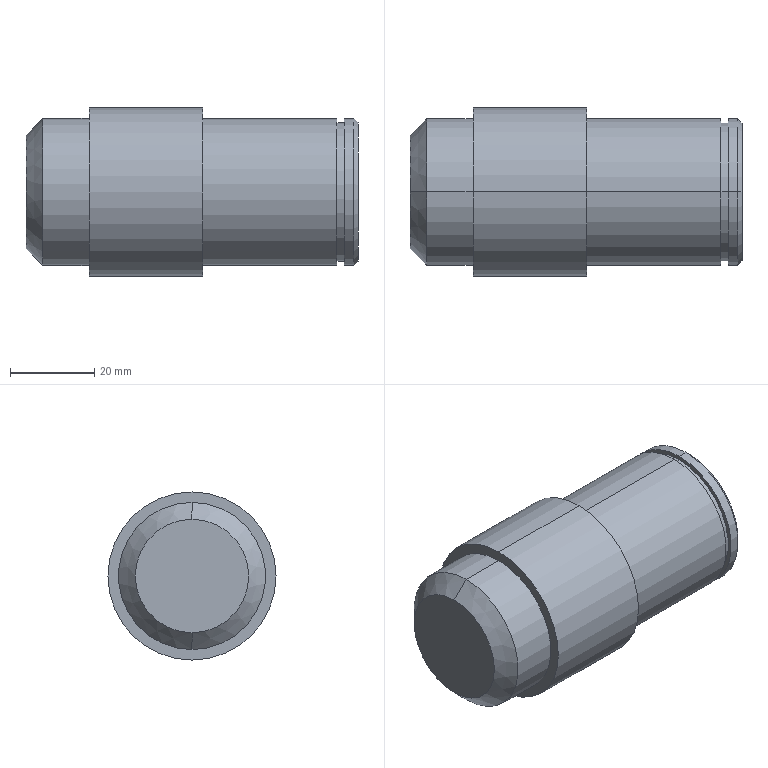Part | STEP file | Driven sprocket shaft | 1 solid | 20 faces | box 79 x 40 x 40 mm | volume 82911 mm3 | cylinder 10 | plane 6 | cone 4 | commonest cylinder face diameters 35 x6 33 x2 40 x2
STEP:
#1=CARTESIAN_POINT('',(0.,0.,0.));
#2=DIRECTION('',(0.,0.,1.));
#3=DIRECTION('',(1.,0.,0.));
#4=AXIS2_PLACEMENT_3D('',#1,#2,#3);
#5=CARTESIAN_POINT('',(0.,0.,13.5));
#6=VERTEX_POINT('',#5);
#7=CARTESIAN_POINT('',(0.,0.,-13.5));
#8=VERTEX_POINT('',#7);
#9=CARTESIAN_POINT('',(0.,0.,0.));
#10=DIRECTION('',(-1.,0.,0.));
#11=DIRECTION('',(0.,0.,-1.));
#12=AXIS2_PLACEMENT_3D('',#9,#10,#11);
#13=CIRCLE('',#12,13.5);
#14=CARTESIAN_POINT('',(0.,0.,0.));
#15=DIRECTION('',(1.,0.,0.));
#16=DIRECTION('',(0.,0.,-1.));
#17=AXIS2_PLACEMENT_3D('',#14,#15,#16);
#18=CONICAL_SURFACE('',#17,13.5,0.7854);
#19=CARTESIAN_POINT('',(6.283,0.));
#20=DIRECTION('',(-1.,0.));
#21=VECTOR('',#20,1.);
#22=LINE('',#19,#21);
#23=(GEOMETRIC_REPRESENTATION_CONTEXT(2)PARAMETRIC_REPRESENTATION_CONTEXT()REPRESENTATION_CONTEXT('',''));
#24=DEFINITIONAL_REPRESENTATION('',(#22),#23);
#25=PCURVE('',#18,#24);
#26=CARTESIAN_POINT('',(0.,0.,0.));
#27=DIRECTION('',(1.,0.,0.));
#28=DIRECTION('',(0.,0.,-1.));
#29=AXIS2_PLACEMENT_3D('',#26,#27,#28);
#30=PLANE('',#29);
#31=CARTESIAN_POINT('',(13.5,0.));
#32=CARTESIAN_POINT('',(13.5,-23.383));
#33=CARTESIAN_POINT('',(-6.75,-11.691));
#34=CARTESIAN_POINT('',(-27.,0.));
#35=CARTESIAN_POINT('',(-6.75,11.691));
#36=CARTESIAN_POINT('',(13.5,23.383));
#37=CARTESIAN_POINT('',(13.5,0.));
#38=(BOUNDED_CURVE()B_SPLINE_CURVE(2,(#31,#32,#33,#34,#35,#36,#37),.UNSPECIFIED.,.T.,.F.)B_SPLINE_CURVE_WITH_KNOTS((1,2,2,2,2,1),(-2.094,0.,2.094,4.189,6.283,8.378),.UNSPECIFIED.)CURVE()GEOMETRIC_REPRESENTATION_ITEM()RATIONAL_B_SPLINE_CURVE((1.,0.5,1.,0.5,1.,0.5,1.))REPRESENTATION_ITEM(''));
#39=(GEOMETRIC_REPRESENTATION_CONTEXT(2)PARAMETRIC_REPRESENTATION_CONTEXT()REPRESENTATION_CONTEXT('',''));
#40=DEFINITIONAL_REPRESENTATION('',(#38),#39);
#41=PCURVE('',#30,#40);
#42=SURFACE_CURVE('',#13,(#25,#41),.PCURVE_S1.);
#43=EDGE_CURVE('',#6,#8,#42,.T.);
#44=ORIENTED_EDGE('',*,*,#43,.F.);
#45=CARTESIAN_POINT('',(4.,0.,17.5));
#46=VERTEX_POINT('',#45);
#47=CARTESIAN_POINT('',(0.,0.,13.5));
#48=DIRECTION('',(0.7071,0.,0.7071));
#49=VECTOR('',#48,1.);
#50=LINE('',#47,#49);
#51=CARTESIAN_POINT('',(3.142,0.));
#52=DIRECTION('',(0.,1.));
#53=VECTOR('',#52,1.);
#54=LINE('',#51,#53);
#55=(GEOMETRIC_REPRESENTATION_CONTEXT(2)PARAMETRIC_REPRESENTATION_CONTEXT()REPRESENTATION_CONTEXT('',''));
#56=DEFINITIONAL_REPRESENTATION('',(#54),#55);
#57=PCURVE('',#18,#56);
#58=CARTESIAN_POINT('',(0.,0.,0.));
#59=DIRECTION('',(1.,0.,0.));
#60=DIRECTION('',(0.,0.,-1.));
#61=AXIS2_PLACEMENT_3D('',#58,#59,#60);
#62=CONICAL_SURFACE('',#61,13.5,0.7854);
#63=CARTESIAN_POINT('',(3.142,0.));
#64=DIRECTION('',(0.,1.));
#65=VECTOR('',#64,1.);
#66=LINE('',#63,#65);
#67=(GEOMETRIC_REPRESENTATION_CONTEXT(2)PARAMETRIC_REPRESENTATION_CONTEXT()REPRESENTATION_CONTEXT('',''));
#68=DEFINITIONAL_REPRESENTATION('',(#66),#67);
#69=PCURVE('',#62,#68);
#70=SURFACE_CURVE('',#50,(#57,#69),.PCURVE_S1.);
#71=EDGE_CURVE('',#6,#46,#70,.T.);
#72=ORIENTED_EDGE('',*,*,#71,.T.);
#73=CARTESIAN_POINT('',(4.,0.,-17.5));
#74=VERTEX_POINT('',#73);
#75=CARTESIAN_POINT('',(4.,0.,0.));
#76=DIRECTION('',(1.,0.,0.));
#77=DIRECTION('',(0.,0.,-1.));
#78=AXIS2_PLACEMENT_3D('',#75,#76,#77);
#79=CIRCLE('',#78,17.5);
#80=CARTESIAN_POINT('',(0.,4.));
#81=DIRECTION('',(1.,0.));
#82=VECTOR('',#81,1.);
#83=LINE('',#80,#82);
#84=(GEOMETRIC_REPRESENTATION_CONTEXT(2)PARAMETRIC_REPRESENTATION_CONTEXT()REPRESENTATION_CONTEXT('',''));
#85=DEFINITIONAL_REPRESENTATION('',(#83),#84);
#86=PCURVE('',#18,#85);
#87=CARTESIAN_POINT('',(-1000.,0.,0.));
#88=DIRECTION('',(-1.,0.,0.));
#89=DIRECTION('',(0.,0.,1.));
#90=AXIS2_PLACEMENT_3D('',#87,#88,#89);
#91=CYLINDRICAL_SURFACE('',#90,17.5);
#92=CARTESIAN_POINT('',(3.142,-1004.));
#93=DIRECTION('',(-1.,0.));
#94=VECTOR('',#93,1.);
#95=LINE('',#92,#94);
#96=(GEOMETRIC_REPRESENTATION_CONTEXT(2)PARAMETRIC_REPRESENTATION_CONTEXT()REPRESENTATION_CONTEXT('',''));
#97=DEFINITIONAL_REPRESENTATION('',(#95),#96);
#98=PCURVE('',#91,#97);
#99=SURFACE_CURVE('',#79,(#86,#98),.PCURVE_S1.);
#100=EDGE_CURVE('',#74,#46,#99,.T.);
#101=ORIENTED_EDGE('',*,*,#100,.F.);
#102=CARTESIAN_POINT('',(0.,0.,-13.5));
#103=DIRECTION('',(0.7071,0.,-0.7071));
#104=VECTOR('',#103,1.);
#105=LINE('',#102,#104);
#106=CARTESIAN_POINT('',(0.,0.));
#107=DIRECTION('',(0.,1.));
#108=VECTOR('',#107,1.);
#109=LINE('',#106,#108);
#110=(GEOMETRIC_REPRESENTATION_CONTEXT(2)PARAMETRIC_REPRESENTATION_CONTEXT()REPRESENTATION_CONTEXT('',''));
#111=DEFINITIONAL_REPRESENTATION('',(#109),#110);
#112=PCURVE('',#18,#111);
#113=CARTESIAN_POINT('',(6.283,0.));
#114=DIRECTION('',(0.,1.));
#115=VECTOR('',#114,1.);
#116=LINE('',#113,#115);
#117=(GEOMETRIC_REPRESENTATION_CONTEXT(2)PARAMETRIC_REPRESENTATION_CONTEXT()REPRESENTATION_CONTEXT('',''));
#118=DEFINITIONAL_REPRESENTATION('',(#116),#117);
#119=PCURVE('',#62,#118);
#120=SURFACE_CURVE('',#105,(#112,#119),.PCURVE_S1.);
#121=EDGE_CURVE('',#8,#74,#120,.T.);
#122=ORIENTED_EDGE('',*,*,#121,.F.);
#123=EDGE_LOOP('',(#44,#72,#101,#122));
#124=FACE_BOUND('',#123,.T.);
#125=ADVANCED_FACE('',(#124),#18,.T.);
#126=CARTESIAN_POINT('',(79.,0.,-16.5));
#127=VERTEX_POINT('',#126);
#128=CARTESIAN_POINT('',(79.,0.,16.5));
#129=VERTEX_POINT('',#128);
#130=CARTESIAN_POINT('',(79.,0.,0.));
#131=DIRECTION('',(1.,0.,0.));
#132=DIRECTION('',(0.,0.,1.));
#133=AXIS2_PLACEMENT_3D('',#130,#131,#132);
#134=CIRCLE('',#133,16.5);
#135=CARTESIAN_POINT('',(78.,0.,0.));
#136=DIRECTION('',(-1.,0.,0.));
#137=DIRECTION('',(0.,0.,1.));
#138=AXIS2_PLACEMENT_3D('',#135,#136,#137);
#139=CONICAL_SURFACE('',#138,17.5,0.7854);
#140=CARTESIAN_POINT('',(6.283,-1.));
#141=DIRECTION('',(-1.,0.));
#142=VECTOR('',#141,1.);
#143=LINE('',#140,#142);
#144=(GEOMETRIC_REPRESENTATION_CONTEXT(2)PARAMETRIC_REPRESENTATION_CONTEXT()REPRESENTATION_CONTEXT('',''));
#145=DEFINITIONAL_REPRESENTATION('',(#143),#144);
#146=PCURVE('',#139,#145);
#147=CARTESIAN_POINT('',(79.,17.5,0.));
#148=DIRECTION('',(-1.,0.,0.));
#149=DIRECTION('',(0.,0.,1.));
#150=AXIS2_PLACEMENT_3D('',#147,#148,#149);
#151=PLANE('',#150);
#152=CARTESIAN_POINT('',(16.5,-17.5));
#153=CARTESIAN_POINT('',(16.5,-46.079));
#154=CARTESIAN_POINT('',(-8.25,-31.789));
#155=CARTESIAN_POINT('',(-33.,-17.5));
#156=CARTESIAN_POINT('',(-8.25,-3.211));
#157=CARTESIAN_POINT('',(16.5,11.079));
#158=CARTESIAN_POINT('',(16.5,-17.5));
#159=(BOUNDED_CURVE()B_SPLINE_CURVE(2,(#152,#153,#154,#155,#156,#157,#158),.UNSPECIFIED.,.T.,.F.)B_SPLINE_CURVE_WITH_KNOTS((1,2,2,2,2,1),(-2.094,0.,2.094,4.189,6.283,8.378),.UNSPECIFIED.)CURVE()GEOMETRIC_REPRESENTATION_ITEM()RATIONAL_B_SPLINE_CURVE((1.,0.5,1.,0.5,1.,0.5,1.))REPRESENTATION_ITEM(''));
#160=(GEOMETRIC_REPRESENTATION_CONTEXT(2)PARAMETRIC_REPRESENTATION_CONTEXT()REPRESENTATION_CONTEXT('',''));
#161=DEFINITIONAL_REPRESENTATION('',(#159),#160);
#162=PCURVE('',#151,#161);
#163=SURFACE_CURVE('',#134,(#146,#162),.PCURVE_S1.);
#164=EDGE_CURVE('',#127,#129,#163,.T.);
#165=ORIENTED_EDGE('',*,*,#164,.F.);
#166=CARTESIAN_POINT('',(78.,0.,-17.5));
#167=VERTEX_POINT('',#166);
#168=CARTESIAN_POINT('',(78.,0.,-17.5));
#169=DIRECTION('',(-0.7071,0.,-0.7071));
#170=VECTOR('',#169,1.);
#171=LINE('',#168,#170);
#172=CARTESIAN_POINT('',(3.142,0.));
#173=DIRECTION('',(0.,1.));
#174=VECTOR('',#173,1.);
#175=LINE('',#172,#174);
#176=(GEOMETRIC_REPRESENTATION_CONTEXT(2)PARAMETRIC_REPRESENTATION_CONTEXT()REPRESENTATION_CONTEXT('',''));
#177=DEFINITIONAL_REPRESENTATION('',(#175),#176);
#178=PCURVE('',#139,#177);
#179=CARTESIAN_POINT('',(78.,0.,0.));
#180=DIRECTION('',(-1.,0.,0.));
#181=DIRECTION('',(0.,0.,1.));
#182=AXIS2_PLACEMENT_3D('',#179,#180,#181);
#183=CONICAL_SURFACE('',#182,17.5,0.7854);
#184=CARTESIAN_POINT('',(3.142,0.));
#185=DIRECTION('',(0.,1.));
#186=VECTOR('',#185,1.);
#187=LINE('',#184,#186);
#188=(GEOMETRIC_REPRESENTATION_CONTEXT(2)PARAMETRIC_REPRESENTATION_CONTEXT()REPRESENTATION_CONTEXT('',''));
#189=DEFINITIONAL_REPRESENTATION('',(#187),#188);
#190=PCURVE('',#183,#189);
#191=SURFACE_CURVE('',#171,(#178,#190),.PCURVE_S1.);
#192=EDGE_CURVE('',#127,#167,#191,.T.);
#193=ORIENTED_EDGE('',*,*,#192,.T.);
#194=CARTESIAN_POINT('',(78.,0.,17.5));
#195=VERTEX_POINT('',#194);
#196=CARTESIAN_POINT('',(78.,0.,0.));
#197=DIRECTION('',(-1.,0.,0.));
#198=DIRECTION('',(0.,0.,1.));
#199=AXIS2_PLACEMENT_3D('',#196,#197,#198);
#200=CIRCLE('',#199,17.5);
#201=CARTESIAN_POINT('',(0.,0.));
#202=DIRECTION('',(1.,0.));
#203=VECTOR('',#202,1.);
#204=LINE('',#201,#203);
#205=(GEOMETRIC_REPRESENTATION_CONTEXT(2)PARAMETRIC_REPRESENTATION_CONTEXT()REPRESENTATION_CONTEXT('',''));
#206=DEFINITIONAL_REPRESENTATION('',(#204),#205);
#207=PCURVE('',#139,#206);
#208=CARTESIAN_POINT('',(-1000.,0.,0.));
#209=DIRECTION('',(-1.,0.,0.));
#210=DIRECTION('',(0.,0.,1.));
#211=AXIS2_PLACEMENT_3D('',#208,#209,#210);
#212=CYLINDRICAL_SURFACE('',#211,17.5);
#213=CARTESIAN_POINT('',(0.,-1078.));
#214=DIRECTION('',(1.,0.));
#215=VECTOR('',#214,1.);
#216=LINE('',#213,#215);
#217=(GEOMETRIC_REPRESENTATION_CONTEXT(2)PARAMETRIC_REPRESENTATION_CONTEXT()REPRESENTATION_CONTEXT('',''));
#218=DEFINITIONAL_REPRESENTATION('',(#216),#217);
#219=PCURVE('',#212,#218);
#220=SURFACE_CURVE('',#200,(#207,#219),.PCURVE_S1.);
#221=EDGE_CURVE('',#195,#167,#220,.T.);
#222=ORIENTED_EDGE('',*,*,#221,.F.);
#223=CARTESIAN_POINT('',(78.,0.,17.5));
#224=DIRECTION('',(-0.7071,0.,0.7071));
#225=VECTOR('',#224,1.);
#226=LINE('',#223,#225);
#227=CARTESIAN_POINT('',(0.,0.));
#228=DIRECTION('',(0.,1.));
#229=VECTOR('',#228,1.);
#230=LINE('',#227,#229);
#231=(GEOMETRIC_REPRESENTATION_CONTEXT(2)PARAMETRIC_REPRESENTATION_CONTEXT()REPRESENTATION_CONTEXT('',''));
#232=DEFINITIONAL_REPRESENTATION('',(#230),#231);
#233=PCURVE('',#139,#232);
#234=CARTESIAN_POINT('',(6.283,0.));
#235=DIRECTION('',(0.,1.));
#236=VECTOR('',#235,1.);
#237=LINE('',#234,#236);
#238=(GEOMETRIC_REPRESENTATION_CONTEXT(2)PARAMETRIC_REPRESENTATION_CONTEXT()REPRESENTATION_CONTEXT('',''));
#239=DEFINITIONAL_REPRESENTATION('',(#237),#238);
#240=PCURVE('',#183,#239);
#241=SURFACE_CURVE('',#226,(#233,#240),.PCURVE_S1.);
#242=EDGE_CURVE('',#129,#195,#241,.T.);
#243=ORIENTED_EDGE('',*,*,#242,.F.);
#244=EDGE_LOOP('',(#165,#193,#222,#243));
#245=FACE_BOUND('',#244,.T.);
#246=ADVANCED_FACE('',(#245),#139,.T.);
#247=ORIENTED_EDGE('',*,*,#221,.T.);
#248=CARTESIAN_POINT('',(75.7,0.,-17.5));
#249=VERTEX_POINT('',#248);
#250=CARTESIAN_POINT('',(-1000.,0.,-17.5));
#251=DIRECTION('',(-1.,0.,0.));
#252=VECTOR('',#251,1.);
#253=LINE('',#250,#252);
#254=CARTESIAN_POINT('',(3.142,0.));
#255=DIRECTION('',(0.,1.));
#256=VECTOR('',#255,1.);
#257=LINE('',#254,#256);
#258=(GEOMETRIC_REPRESENTATION_CONTEXT(2)PARAMETRIC_REPRESENTATION_CONTEXT()REPRESENTATION_CONTEXT('',''));
#259=DEFINITIONAL_REPRESENTATION('',(#257),#258);
#260=PCURVE('',#212,#259);
#261=CARTESIAN_POINT('',(-1000.,0.,0.));
#262=DIRECTION('',(-1.,0.,0.));
#263=DIRECTION('',(0.,0.,1.));
#264=AXIS2_PLACEMENT_3D('',#261,#262,#263);
#265=CYLINDRICAL_SURFACE('',#264,17.5);
#266=CARTESIAN_POINT('',(3.142,0.));
#267=DIRECTION('',(0.,1.));
#268=VECTOR('',#267,1.);
#269=LINE('',#266,#268);
#270=(GEOMETRIC_REPRESENTATION_CONTEXT(2)PARAMETRIC_REPRESENTATION_CONTEXT()REPRESENTATION_CONTEXT('',''));
#271=DEFINITIONAL_REPRESENTATION('',(#269),#270);
#272=PCURVE('',#265,#271);
#273=SURFACE_CURVE('',#253,(#260,#272),.PCURVE_S1.);
#274=EDGE_CURVE('',#167,#249,#273,.T.);
#275=ORIENTED_EDGE('',*,*,#274,.T.);
#276=CARTESIAN_POINT('',(75.7,0.,17.5));
#277=VERTEX_POINT('',#276);
#278=CARTESIAN_POINT('',(75.7,0.,0.));
#279=DIRECTION('',(-1.,0.,0.));
#280=DIRECTION('',(0.,0.,1.));
#281=AXIS2_PLACEMENT_3D('',#278,#279,#280);
#282=CIRCLE('',#281,17.5);
#283=CARTESIAN_POINT('',(0.,-1075.7));
#284=DIRECTION('',(1.,0.));
#285=VECTOR('',#284,1.);
#286=LINE('',#283,#285);
#287=(GEOMETRIC_REPRESENTATION_CONTEXT(2)PARAMETRIC_REPRESENTATION_CONTEXT()REPRESENTATION_CONTEXT('',''));
#288=DEFINITIONAL_REPRESENTATION('',(#286),#287);
#289=PCURVE('',#212,#288);
#290=CARTESIAN_POINT('',(75.7,16.5,0.));
#291=DIRECTION('',(1.,0.,0.));
#292=DIRECTION('',(0.,0.,-1.));
#293=AXIS2_PLACEMENT_3D('',#290,#291,#292);
#294=PLANE('',#293);
#295=CARTESIAN_POINT('',(-17.5,-16.5));
#296=CARTESIAN_POINT('',(-17.5,13.811));
#297=CARTESIAN_POINT('',(8.75,-1.345));
#298=CARTESIAN_POINT('',(35.,-16.5));
#299=CARTESIAN_POINT('',(8.75,-31.655));
#300=CARTESIAN_POINT('',(-17.5,-46.811));
#301=CARTESIAN_POINT('',(-17.5,-16.5));
#302=(BOUNDED_CURVE()B_SPLINE_CURVE(2,(#295,#296,#297,#298,#299,#300,#301),.UNSPECIFIED.,.T.,.F.)B_SPLINE_CURVE_WITH_KNOTS((1,2,2,2,2,1),(-2.094,0.,2.094,4.189,6.283,8.378),.UNSPECIFIED.)CURVE()GEOMETRIC_REPRESENTATION_ITEM()RATIONAL_B_SPLINE_CURVE((1.,0.5,1.,0.5,1.,0.5,1.))REPRESENTATION_ITEM(''));
#303=(GEOMETRIC_REPRESENTATION_CONTEXT(2)PARAMETRIC_REPRESENTATION_CONTEXT()REPRESENTATION_CONTEXT('',''));
#304=DEFINITIONAL_REPRESENTATION('',(#302),#303);
#305=PCURVE('',#294,#304);
#306=SURFACE_CURVE('',#282,(#289,#305),.PCURVE_S1.);
#307=EDGE_CURVE('',#277,#249,#306,.T.);
#308=ORIENTED_EDGE('',*,*,#307,.F.);
#309=CARTESIAN_POINT('',(-1000.,0.,17.5));
#310=DIRECTION('',(-1.,0.,0.));
#311=VECTOR('',#310,1.);
#312=LINE('',#309,#311);
#313=CARTESIAN_POINT('',(0.,0.));
#314=DIRECTION('',(0.,1.));
#315=VECTOR('',#314,1.);
#316=LINE('',#313,#315);
#317=(GEOMETRIC_REPRESENTATION_CONTEXT(2)PARAMETRIC_REPRESENTATION_CONTEXT()REPRESENTATION_CONTEXT('',''));
#318=DEFINITIONAL_REPRESENTATION('',(#316),#317);
#319=PCURVE('',#212,#318);
#320=CARTESIAN_POINT('',(6.283,0.));
#321=DIRECTION('',(0.,1.));
#322=VECTOR('',#321,1.);
#323=LINE('',#320,#322);
#324=(GEOMETRIC_REPRESENTATION_CONTEXT(2)PARAMETRIC_REPRESENTATION_CONTEXT()REPRESENTATION_CONTEXT('',''));
#325=DEFINITIONAL_REPRESENTATION('',(#323),#324);
#326=PCURVE('',#265,#325);
#327=SURFACE_CURVE('',#312,(#319,#326),.PCURVE_S1.);
#328=EDGE_CURVE('',#195,#277,#327,.T.);
#329=ORIENTED_EDGE('',*,*,#328,.F.);
#330=EDGE_LOOP('',(#247,#275,#308,#329));
#331=FACE_BOUND('',#330,.T.);
#332=ADVANCED_FACE('',(#331),#212,.T.);
#333=CARTESIAN_POINT('',(75.7,0.,16.5));
#334=VERTEX_POINT('',#333);
#335=CARTESIAN_POINT('',(75.7,0.,-16.5));
#336=VERTEX_POINT('',#335);
#337=CARTESIAN_POINT('',(75.7,0.,0.));
#338=DIRECTION('',(-1.,0.,0.));
#339=DIRECTION('',(0.,0.,1.));
#340=AXIS2_PLACEMENT_3D('',#337,#338,#339);
#341=CIRCLE('',#340,16.5);
#342=CARTESIAN_POINT('',(-1000.,0.,0.));
#343=DIRECTION('',(-1.,0.,0.));
#344=DIRECTION('',(0.,0.,1.));
#345=AXIS2_PLACEMENT_3D('',#342,#343,#344);
#346=CYLINDRICAL_SURFACE('',#345,16.5);
#347=CARTESIAN_POINT('',(0.,-1075.7));
#348=DIRECTION('',(1.,0.));
#349=VECTOR('',#348,1.);
#350=LINE('',#347,#349);
#351=(GEOMETRIC_REPRESENTATION_CONTEXT(2)PARAMETRIC_REPRESENTATION_CONTEXT()REPRESENTATION_CONTEXT('',''));
#352=DEFINITIONAL_REPRESENTATION('',(#350),#351);
#353=PCURVE('',#346,#352);
#354=CARTESIAN_POINT('',(-16.5,-16.5));
#355=CARTESIAN_POINT('',(-16.5,12.079));
#356=CARTESIAN_POINT('',(8.25,-2.211));
#357=CARTESIAN_POINT('',(33.,-16.5));
#358=CARTESIAN_POINT('',(8.25,-30.789));
#359=CARTESIAN_POINT('',(-16.5,-45.079));
#360=CARTESIAN_POINT('',(-16.5,-16.5));
#361=(BOUNDED_CURVE()B_SPLINE_CURVE(2,(#354,#355,#356,#357,#358,#359,#360),.UNSPECIFIED.,.T.,.F.)B_SPLINE_CURVE_WITH_KNOTS((1,2,2,2,2,1),(-2.094,0.,2.094,4.189,6.283,8.378),.UNSPECIFIED.)CURVE()GEOMETRIC_REPRESENTATION_ITEM()RATIONAL_B_SPLINE_CURVE((1.,0.5,1.,0.5,1.,0.5,1.))REPRESENTATION_ITEM(''));
#362=(GEOMETRIC_REPRESENTATION_CONTEXT(2)PARAMETRIC_REPRESENTATION_CONTEXT()REPRESENTATION_CONTEXT('',''));
#363=DEFINITIONAL_REPRESENTATION('',(#361),#362);
#364=PCURVE('',#294,#363);
#365=SURFACE_CURVE('',#341,(#353,#364),.PCURVE_S1.);
#366=EDGE_CURVE('',#334,#336,#365,.T.);
#367=ORIENTED_EDGE('',*,*,#366,.T.);
#368=CARTESIAN_POINT('',(74.,0.,-16.5));
#369=VERTEX_POINT('',#368);
#370=CARTESIAN_POINT('',(-1000.,0.,-16.5));
#371=DIRECTION('',(-1.,0.,0.));
#372=VECTOR('',#371,1.);
#373=LINE('',#370,#372);
#374=CARTESIAN_POINT('',(3.142,0.));
#375=DIRECTION('',(0.,1.));
#376=VECTOR('',#375,1.);
#377=LINE('',#374,#376);
#378=(GEOMETRIC_REPRESENTATION_CONTEXT(2)PARAMETRIC_REPRESENTATION_CONTEXT()REPRESENTATION_CONTEXT('',''));
#379=DEFINITIONAL_REPRESENTATION('',(#377),#378);
#380=PCURVE('',#346,#379);
#381=CARTESIAN_POINT('',(-1000.,0.,0.));
#382=DIRECTION('',(-1.,0.,0.));
#383=DIRECTION('',(0.,0.,1.));
#384=AXIS2_PLACEMENT_3D('',#381,#382,#383);
#385=CYLINDRICAL_SURFACE('',#384,16.5);
#386=CARTESIAN_POINT('',(3.142,0.));
#387=DIRECTION('',(0.,1.));
#388=VECTOR('',#387,1.);
#389=LINE('',#386,#388);
#390=(GEOMETRIC_REPRESENTATION_CONTEXT(2)PARAMETRIC_REPRESENTATION_CONTEXT()REPRESENTATION_CONTEXT('',''));
#391=DEFINITIONAL_REPRESENTATION('',(#389),#390);
#392=PCURVE('',#385,#391);
#393=SURFACE_CURVE('',#373,(#380,#392),.PCURVE_S1.);
#394=EDGE_CURVE('',#336,#369,#393,.T.);
#395=ORIENTED_EDGE('',*,*,#394,.T.);
#396=CARTESIAN_POINT('',(74.,0.,16.5));
#397=VERTEX_POINT('',#396);
#398=CARTESIAN_POINT('',(74.,0.,0.));
#399=DIRECTION('',(-1.,0.,0.));
#400=DIRECTION('',(0.,0.,1.));
#401=AXIS2_PLACEMENT_3D('',#398,#399,#400);
#402=CIRCLE('',#401,16.5);
#403=CARTESIAN_POINT('',(0.,-1074.));
#404=DIRECTION('',(1.,0.));
#405=VECTOR('',#404,1.);
#406=LINE('',#403,#405);
#407=(GEOMETRIC_REPRESENTATION_CONTEXT(2)PARAMETRIC_REPRESENTATION_CONTEXT()REPRESENTATION_CONTEXT('',''));
#408=DEFINITIONAL_REPRESENTATION('',(#406),#407);
#409=PCURVE('',#346,#408);
#410=CARTESIAN_POINT('',(74.,17.5,0.));
#411=DIRECTION('',(-1.,0.,0.));
#412=DIRECTION('',(0.,0.,1.));
#413=AXIS2_PLACEMENT_3D('',#410,#411,#412);
#414=PLANE('',#413);
#415=CARTESIAN_POINT('',(0.,-17.5));
#416=DIRECTION('',(1.,0.));
#417=AXIS2_PLACEMENT_2D('',#415,#416);
#418=CIRCLE('',#417,16.5);
#419=(GEOMETRIC_REPRESENTATION_CONTEXT(2)PARAMETRIC_REPRESENTATION_CONTEXT()REPRESENTATION_CONTEXT('',''));
#420=DEFINITIONAL_REPRESENTATION('',(#418),#419);
#421=PCURVE('',#414,#420);
#422=SURFACE_CURVE('',#402,(#409,#421),.PCURVE_S1.);
#423=EDGE_CURVE('',#397,#369,#422,.T.);
#424=ORIENTED_EDGE('',*,*,#423,.F.);
#425=CARTESIAN_POINT('',(-1000.,0.,16.5));
#426=DIRECTION('',(-1.,0.,0.));
#427=VECTOR('',#426,1.);
#428=LINE('',#425,#427);
#429=CARTESIAN_POINT('',(0.,0.));
#430=DIRECTION('',(0.,1.));
#431=VECTOR('',#430,1.);
#432=LINE('',#429,#431);
#433=(GEOMETRIC_REPRESENTATION_CONTEXT(2)PARAMETRIC_REPRESENTATION_CONTEXT()REPRESENTATION_CONTEXT('',''));
#434=DEFINITIONAL_REPRESENTATION('',(#432),#433);
#435=PCURVE('',#346,#434);
#436=CARTESIAN_POINT('',(6.283,0.));
#437=DIRECTION('',(0.,1.));
#438=VECTOR('',#437,1.);
#439=LINE('',#436,#438);
#440=(GEOMETRIC_REPRESENTATION_CONTEXT(2)PARAMETRIC_REPRESENTATION_CONTEXT()REPRESENTATION_CONTEXT('',''));
#441=DEFINITIONAL_REPRESENTATION('',(#439),#440);
#442=PCURVE('',#385,#441);
#443=SURFACE_CURVE('',#428,(#435,#442),.PCURVE_S1.);
#444=EDGE_CURVE('',#334,#397,#443,.T.);
#445=ORIENTED_EDGE('',*,*,#444,.F.);
#446=EDGE_LOOP('',(#367,#395,#424,#445));
#447=FACE_BOUND('',#446,.T.);
#448=ADVANCED_FACE('',(#447),#346,.T.);
#449=CARTESIAN_POINT('',(74.,0.,17.5));
#450=VERTEX_POINT('',#449);
#451=CARTESIAN_POINT('',(74.,0.,-17.5));
#452=VERTEX_POINT('',#451);
#453=CARTESIAN_POINT('',(74.,0.,0.));
#454=DIRECTION('',(-1.,0.,0.));
#455=DIRECTION('',(0.,0.,1.));
#456=AXIS2_PLACEMENT_3D('',#453,#454,#455);
#457=CIRCLE('',#456,17.5);
#458=CARTESIAN_POINT('',(-1000.,0.,0.));
#459=DIRECTION('',(-1.,0.,0.));
#460=DIRECTION('',(0.,0.,1.));
#461=AXIS2_PLACEMENT_3D('',#458,#459,#460);
#462=CYLINDRICAL_SURFACE('',#461,17.5);
#463=CARTESIAN_POINT('',(0.,-1074.));
#464=DIRECTION('',(1.,0.));
#465=VECTOR('',#464,1.);
#466=LINE('',#463,#465);
#467=(GEOMETRIC_REPRESENTATION_CONTEXT(2)PARAMETRIC_REPRESENTATION_CONTEXT()REPRESENTATION_CONTEXT('',''));
#468=DEFINITIONAL_REPRESENTATION('',(#466),#467);
#469=PCURVE('',#462,#468);
#470=CARTESIAN_POINT('',(0.,-17.5));
#471=DIRECTION('',(1.,0.));
#472=AXIS2_PLACEMENT_2D('',#470,#471);
#473=CIRCLE('',#472,17.5);
#474=(GEOMETRIC_REPRESENTATION_CONTEXT(2)PARAMETRIC_REPRESENTATION_CONTEXT()REPRESENTATION_CONTEXT('',''));
#475=DEFINITIONAL_REPRESENTATION('',(#473),#474);
#476=PCURVE('',#414,#475);
#477=SURFACE_CURVE('',#457,(#469,#476),.PCURVE_S1.);
#478=EDGE_CURVE('',#450,#452,#477,.T.);
#479=ORIENTED_EDGE('',*,*,#478,.T.);
#480=CARTESIAN_POINT('',(42.,0.,-17.5));
#481=VERTEX_POINT('',#480);
#482=CARTESIAN_POINT('',(-1000.,0.,-17.5));
#483=DIRECTION('',(-1.,0.,0.));
#484=VECTOR('',#483,1.);
#485=LINE('',#482,#484);
#486=CARTESIAN_POINT('',(3.142,0.));
#487=DIRECTION('',(0.,1.));
#488=VECTOR('',#487,1.);
#489=LINE('',#486,#488);
#490=(GEOMETRIC_REPRESENTATION_CONTEXT(2)PARAMETRIC_REPRESENTATION_CONTEXT()REPRESENTATION_CONTEXT('',''));
#491=DEFINITIONAL_REPRESENTATION('',(#489),#490);
#492=PCURVE('',#462,#491);
#493=CARTESIAN_POINT('',(-1000.,0.,0.));
#494=DIRECTION('',(-1.,0.,0.));
#495=DIRECTION('',(0.,0.,1.));
#496=AXIS2_PLACEMENT_3D('',#493,#494,#495);
#497=CYLINDRICAL_SURFACE('',#496,17.5);
#498=CARTESIAN_POINT('',(3.142,0.));
#499=DIRECTION('',(0.,1.));
#500=VECTOR('',#499,1.);
#501=LINE('',#498,#500);
#502=(GEOMETRIC_REPRESENTATION_CONTEXT(2)PARAMETRIC_REPRESENTATION_CONTEXT()REPRESENTATION_CONTEXT('',''));
#503=DEFINITIONAL_REPRESENTATION('',(#501),#502);
#504=PCURVE('',#497,#503);
#505=SURFACE_CURVE('',#485,(#492,#504),.PCURVE_S1.);
#506=EDGE_CURVE('',#452,#481,#505,.T.);
#507=ORIENTED_EDGE('',*,*,#506,.T.);
#508=CARTESIAN_POINT('',(42.,0.,17.5));
#509=VERTEX_POINT('',#508);
#510=CARTESIAN_POINT('',(42.,0.,0.));
#511=DIRECTION('',(-1.,0.,0.));
#512=DIRECTION('',(0.,0.,1.));
#513=AXIS2_PLACEMENT_3D('',#510,#511,#512);
#514=CIRCLE('',#513,17.5);
#515=CARTESIAN_POINT('',(0.,-1042.));
#516=DIRECTION('',(1.,0.));
#517=VECTOR('',#516,1.);
#518=LINE('',#515,#517);
#519=(GEOMETRIC_REPRESENTATION_CONTEXT(2)PARAMETRIC_REPRESENTATION_CONTEXT()REPRESENTATION_CONTEXT('',''));
#520=DEFINITIONAL_REPRESENTATION('',(#518),#519);
#521=PCURVE('',#462,#520);
#522=CARTESIAN_POINT('',(42.,20.,0.));
#523=DIRECTION('',(-1.,0.,0.));
#524=DIRECTION('',(0.,0.,1.));
#525=AXIS2_PLACEMENT_3D('',#522,#523,#524);
#526=PLANE('',#525);
#527=CARTESIAN_POINT('',(0.,-20.));
#528=DIRECTION('',(1.,0.));
#529=AXIS2_PLACEMENT_2D('',#527,#528);
#530=CIRCLE('',#529,17.5);
#531=(GEOMETRIC_REPRESENTATION_CONTEXT(2)PARAMETRIC_REPRESENTATION_CONTEXT()REPRESENTATION_CONTEXT('',''));
#532=DEFINITIONAL_REPRESENTATION('',(#530),#531);
#533=PCURVE('',#526,#532);
#534=SURFACE_CURVE('',#514,(#521,#533),.PCURVE_S1.);
#535=EDGE_CURVE('',#509,#481,#534,.T.);
#536=ORIENTED_EDGE('',*,*,#535,.F.);
#537=CARTESIAN_POINT('',(-1000.,0.,17.5));
#538=DIRECTION('',(-1.,0.,0.));
#539=VECTOR('',#538,1.);
#540=LINE('',#537,#539);
#541=CARTESIAN_POINT('',(0.,0.));
#542=DIRECTION('',(0.,1.));
#543=VECTOR('',#542,1.);
#544=LINE('',#541,#543);
#545=(GEOMETRIC_REPRESENTATION_CONTEXT(2)PARAMETRIC_REPRESENTATION_CONTEXT()REPRESENTATION_CONTEXT('',''));
#546=DEFINITIONAL_REPRESENTATION('',(#544),#545);
#547=PCURVE('',#462,#546);
#548=CARTESIAN_POINT('',(6.283,0.));
#549=DIRECTION('',(0.,1.));
#550=VECTOR('',#549,1.);
#551=LINE('',#548,#550);
#552=(GEOMETRIC_REPRESENTATION_CONTEXT(2)PARAMETRIC_REPRESENTATION_CONTEXT()REPRESENTATION_CONTEXT('',''));
#553=DEFINITIONAL_REPRESENTATION('',(#551),#552);
#554=PCURVE('',#497,#553);
#555=SURFACE_CURVE('',#540,(#547,#554),.PCURVE_S1.);
#556=EDGE_CURVE('',#450,#509,#555,.T.);
#557=ORIENTED_EDGE('',*,*,#556,.F.);
#558=EDGE_LOOP('',(#479,#507,#536,#557));
#559=FACE_BOUND('',#558,.T.);
#560=ADVANCED_FACE('',(#559),#462,.T.);
#561=CARTESIAN_POINT('',(42.,0.,20.));
#562=VERTEX_POINT('',#561);
#563=CARTESIAN_POINT('',(42.,0.,-20.));
#564=VERTEX_POINT('',#563);
#565=CARTESIAN_POINT('',(42.,0.,0.));
#566=DIRECTION('',(-1.,0.,0.));
#567=DIRECTION('',(0.,0.,1.));
#568=AXIS2_PLACEMENT_3D('',#565,#566,#567);
#569=CIRCLE('',#568,20.);
#570=CARTESIAN_POINT('',(-1000.,0.,0.));
#571=DIRECTION('',(-1.,0.,0.));
#572=DIRECTION('',(0.,0.,1.));
#573=AXIS2_PLACEMENT_3D('',#570,#571,#572);
#574=CYLINDRICAL_SURFACE('',#573,20.);
#575=CARTESIAN_POINT('',(0.,-1042.));
#576=DIRECTION('',(1.,0.));
#577=VECTOR('',#576,1.);
#578=LINE('',#575,#577);
#579=(GEOMETRIC_REPRESENTATION_CONTEXT(2)PARAMETRIC_REPRESENTATION_CONTEXT()REPRESENTATION_CONTEXT('',''));
#580=DEFINITIONAL_REPRESENTATION('',(#578),#579);
#581=PCURVE('',#574,#580);
#582=CARTESIAN_POINT('',(0.,-20.));
#583=DIRECTION('',(1.,0.));
#584=AXIS2_PLACEMENT_2D('',#582,#583);
#585=CIRCLE('',#584,20.);
#586=(GEOMETRIC_REPRESENTATION_CONTEXT(2)PARAMETRIC_REPRESENTATION_CONTEXT()REPRESENTATION_CONTEXT('',''));
#587=DEFINITIONAL_REPRESENTATION('',(#585),#586);
#588=PCURVE('',#526,#587);
#589=SURFACE_CURVE('',#569,(#581,#588),.PCURVE_S1.);
#590=EDGE_CURVE('',#562,#564,#589,.T.);
#591=ORIENTED_EDGE('',*,*,#590,.T.);
#592=CARTESIAN_POINT('',(15.,0.,-20.));
#593=VERTEX_POINT('',#592);
#594=CARTESIAN_POINT('',(-1000.,0.,-20.));
#595=DIRECTION('',(-1.,0.,0.));
#596=VECTOR('',#595,1.);
#597=LINE('',#594,#596);
#598=CARTESIAN_POINT('',(3.142,0.));
#599=DIRECTION('',(0.,1.));
#600=VECTOR('',#599,1.);
#601=LINE('',#598,#600);
#602=(GEOMETRIC_REPRESENTATION_CONTEXT(2)PARAMETRIC_REPRESENTATION_CONTEXT()REPRESENTATION_CONTEXT('',''));
#603=DEFINITIONAL_REPRESENTATION('',(#601),#602);
#604=PCURVE('',#574,#603);
#605=CARTESIAN_POINT('',(-1000.,0.,0.));
#606=DIRECTION('',(-1.,0.,0.));
#607=DIRECTION('',(0.,0.,1.));
#608=AXIS2_PLACEMENT_3D('',#605,#606,#607);
#609=CYLINDRICAL_SURFACE('',#608,20.);
#610=CARTESIAN_POINT('',(3.142,0.));
#611=DIRECTION('',(0.,1.));
#612=VECTOR('',#611,1.);
#613=LINE('',#610,#612);
#614=(GEOMETRIC_REPRESENTATION_CONTEXT(2)PARAMETRIC_REPRESENTATION_CONTEXT()REPRESENTATION_CONTEXT('',''));
#615=DEFINITIONAL_REPRESENTATION('',(#613),#614);
#616=PCURVE('',#609,#615);
#617=SURFACE_CURVE('',#597,(#604,#616),.PCURVE_S1.);
#618=EDGE_CURVE('',#564,#593,#617,.T.);
#619=ORIENTED_EDGE('',*,*,#618,.T.);
#620=CARTESIAN_POINT('',(15.,0.,20.));
#621=VERTEX_POINT('',#620);
#622=CARTESIAN_POINT('',(15.,0.,0.));
#623=DIRECTION('',(-1.,0.,0.));
#624=DIRECTION('',(0.,0.,1.));
#625=AXIS2_PLACEMENT_3D('',#622,#623,#624);
#626=CIRCLE('',#625,20.);
#627=CARTESIAN_POINT('',(0.,-1015.));
#628=DIRECTION('',(1.,0.));
#629=VECTOR('',#628,1.);
#630=LINE('',#627,#629);
#631=(GEOMETRIC_REPRESENTATION_CONTEXT(2)PARAMETRIC_REPRESENTATION_CONTEXT()REPRESENTATION_CONTEXT('',''));
#632=DEFINITIONAL_REPRESENTATION('',(#630),#631);
#633=PCURVE('',#574,#632);
#634=CARTESIAN_POINT('',(15.,17.5,0.));
#635=DIRECTION('',(1.,0.,0.));
#636=DIRECTION('',(0.,0.,-1.));
#637=AXIS2_PLACEMENT_3D('',#634,#635,#636);
#638=PLANE('',#637);
#639=CARTESIAN_POINT('',(-20.,-17.5));
#640=CARTESIAN_POINT('',(-20.,17.141));
#641=CARTESIAN_POINT('',(10.,-0.1795));
#642=CARTESIAN_POINT('',(40.,-17.5));
#643=CARTESIAN_POINT('',(10.,-34.821));
#644=CARTESIAN_POINT('',(-20.,-52.141));
#645=CARTESIAN_POINT('',(-20.,-17.5));
#646=(BOUNDED_CURVE()B_SPLINE_CURVE(2,(#639,#640,#641,#642,#643,#644,#645),.UNSPECIFIED.,.T.,.F.)B_SPLINE_CURVE_WITH_KNOTS((1,2,2,2,2,1),(-2.094,0.,2.094,4.189,6.283,8.378),.UNSPECIFIED.)CURVE()GEOMETRIC_REPRESENTATION_ITEM()RATIONAL_B_SPLINE_CURVE((1.,0.5,1.,0.5,1.,0.5,1.))REPRESENTATION_ITEM(''));
#647=(GEOMETRIC_REPRESENTATION_CONTEXT(2)PARAMETRIC_REPRESENTATION_CONTEXT()REPRESENTATION_CONTEXT('',''));
#648=DEFINITIONAL_REPRESENTATION('',(#646),#647);
#649=PCURVE('',#638,#648);
#650=SURFACE_CURVE('',#626,(#633,#649),.PCURVE_S1.);
#651=EDGE_CURVE('',#621,#593,#650,.T.);
#652=ORIENTED_EDGE('',*,*,#651,.F.);
#653=CARTESIAN_POINT('',(-1000.,0.,20.));
#654=DIRECTION('',(-1.,0.,0.));
#655=VECTOR('',#654,1.);
#656=LINE('',#653,#655);
#657=CARTESIAN_POINT('',(0.,0.));
#658=DIRECTION('',(0.,1.));
#659=VECTOR('',#658,1.);
#660=LINE('',#657,#659);
#661=(GEOMETRIC_REPRESENTATION_CONTEXT(2)PARAMETRIC_REPRESENTATION_CONTEXT()REPRESENTATION_CONTEXT('',''));
#662=DEFINITIONAL_REPRESENTATION('',(#660),#661);
#663=PCURVE('',#574,#662);
#664=CARTESIAN_POINT('',(6.283,0.));
#665=DIRECTION('',(0.,1.));
#666=VECTOR('',#665,1.);
#667=LINE('',#664,#666);
#668=(GEOMETRIC_REPRESENTATION_CONTEXT(2)PARAMETRIC_REPRESENTATION_CONTEXT()REPRESENTATION_CONTEXT('',''));
#669=DEFINITIONAL_REPRESENTATION('',(#667),#668);
#670=PCURVE('',#609,#669);
#671=SURFACE_CURVE('',#656,(#663,#670),.PCURVE_S1.);
#672=EDGE_CURVE('',#562,#621,#671,.T.);
#673=ORIENTED_EDGE('',*,*,#672,.F.);
#674=EDGE_LOOP('',(#591,#619,#652,#673));
#675=FACE_BOUND('',#674,.T.);
#676=ADVANCED_FACE('',(#675),#574,.T.);
#677=CARTESIAN_POINT('',(15.,0.,17.5));
#678=VERTEX_POINT('',#677);
#679=CARTESIAN_POINT('',(15.,0.,-17.5));
#680=VERTEX_POINT('',#679);
#681=CARTESIAN_POINT('',(15.,0.,0.));
#682=DIRECTION('',(-1.,0.,0.));
#683=DIRECTION('',(0.,0.,1.));
#684=AXIS2_PLACEMENT_3D('',#681,#682,#683);
#685=CIRCLE('',#684,17.5);
#686=CARTESIAN_POINT('',(0.,-1015.));
#687=DIRECTION('',(1.,0.));
#688=VECTOR('',#687,1.);
#689=LINE('',#686,#688);
#690=(GEOMETRIC_REPRESENTATION_CONTEXT(2)PARAMETRIC_REPRESENTATION_CONTEXT()REPRESENTATION_CONTEXT('',''));
#691=DEFINITIONAL_REPRESENTATION('',(#689),#690);
#692=PCURVE('',#91,#691);
#693=CARTESIAN_POINT('',(-17.5,-17.5));
#694=CARTESIAN_POINT('',(-17.5,12.811));
#695=CARTESIAN_POINT('',(8.75,-2.345));
#696=CARTESIAN_POINT('',(35.,-17.5));
#697=CARTESIAN_POINT('',(8.75,-32.655));
#698=CARTESIAN_POINT('',(-17.5,-47.811));
#699=CARTESIAN_POINT('',(-17.5,-17.5));
#700=(BOUNDED_CURVE()B_SPLINE_CURVE(2,(#693,#694,#695,#696,#697,#698,#699),.UNSPECIFIED.,.T.,.F.)B_SPLINE_CURVE_WITH_KNOTS((1,2,2,2,2,1),(-2.094,0.,2.094,4.189,6.283,8.378),.UNSPECIFIED.)CURVE()GEOMETRIC_REPRESENTATION_ITEM()RATIONAL_B_SPLINE_CURVE((1.,0.5,1.,0.5,1.,0.5,1.))REPRESENTATION_ITEM(''));
#701=(GEOMETRIC_REPRESENTATION_CONTEXT(2)PARAMETRIC_REPRESENTATION_CONTEXT()REPRESENTATION_CONTEXT('',''));
#702=DEFINITIONAL_REPRESENTATION('',(#700),#701);
#703=PCURVE('',#638,#702);
#704=SURFACE_CURVE('',#685,(#692,#703),.PCURVE_S1.);
#705=EDGE_CURVE('',#678,#680,#704,.T.);
#706=ORIENTED_EDGE('',*,*,#705,.T.);
#707=CARTESIAN_POINT('',(-1000.,0.,-17.5));
#708=DIRECTION('',(-1.,0.,0.));
#709=VECTOR('',#708,1.);
#710=LINE('',#707,#709);
#711=CARTESIAN_POINT('',(3.142,0.));
#712=DIRECTION('',(0.,1.));
#713=VECTOR('',#712,1.);
#714=LINE('',#711,#713);
#715=(GEOMETRIC_REPRESENTATION_CONTEXT(2)PARAMETRIC_REPRESENTATION_CONTEXT()REPRESENTATION_CONTEXT('',''));
#716=DEFINITIONAL_REPRESENTATION('',(#714),#715);
#717=PCURVE('',#91,#716);
#718=CARTESIAN_POINT('',(-1000.,0.,0.));
#719=DIRECTION('',(-1.,0.,0.));
#720=DIRECTION('',(0.,0.,1.));
#721=AXIS2_PLACEMENT_3D('',#718,#719,#720);
#722=CYLINDRICAL_SURFACE('',#721,17.5);
#723=CARTESIAN_POINT('',(3.142,0.));
#724=DIRECTION('',(0.,1.));
#725=VECTOR('',#724,1.);
#726=LINE('',#723,#725);
#727=(GEOMETRIC_REPRESENTATION_CONTEXT(2)PARAMETRIC_REPRESENTATION_CONTEXT()REPRESENTATION_CONTEXT('',''));
#728=DEFINITIONAL_REPRESENTATION('',(#726),#727);
#729=PCURVE('',#722,#728);
#730=SURFACE_CURVE('',#710,(#717,#729),.PCURVE_S1.);
#731=EDGE_CURVE('',#680,#74,#730,.T.);
#732=ORIENTED_EDGE('',*,*,#731,.T.);
#733=ORIENTED_EDGE('',*,*,#100,.T.);
#734=CARTESIAN_POINT('',(-1000.,0.,17.5));
#735=DIRECTION('',(-1.,0.,0.));
#736=VECTOR('',#735,1.);
#737=LINE('',#734,#736);
#738=CARTESIAN_POINT('',(0.,0.));
#739=DIRECTION('',(0.,1.));
#740=VECTOR('',#739,1.);
#741=LINE('',#738,#740);
#742=(GEOMETRIC_REPRESENTATION_CONTEXT(2)PARAMETRIC_REPRESENTATION_CONTEXT()REPRESENTATION_CONTEXT('',''));
#743=DEFINITIONAL_REPRESENTATION('',(#741),#742);
#744=PCURVE('',#91,#743);
#745=CARTESIAN_POINT('',(6.283,0.));
#746=DIRECTION('',(0.,1.));
#747=VECTOR('',#746,1.);
#748=LINE('',#745,#747);
#749=(GEOMETRIC_REPRESENTATION_CONTEXT(2)PARAMETRIC_REPRESENTATION_CONTEXT()REPRESENTATION_CONTEXT('',''));
#750=DEFINITIONAL_REPRESENTATION('',(#748),#749);
#751=PCURVE('',#722,#750);
#752=SURFACE_CURVE('',#737,(#744,#751),.PCURVE_S1.);
#753=EDGE_CURVE('',#678,#46,#752,.T.);
#754=ORIENTED_EDGE('',*,*,#753,.F.);
#755=EDGE_LOOP('',(#706,#732,#733,#754));
#756=FACE_BOUND('',#755,.T.);
#757=ADVANCED_FACE('',(#756),#91,.T.);
#758=CARTESIAN_POINT('',(0.,0.,0.));
#759=DIRECTION('',(-1.,0.,0.));
#760=DIRECTION('',(0.,0.,-1.));
#761=AXIS2_PLACEMENT_3D('',#758,#759,#760);
#762=CIRCLE('',#761,13.5);
#763=CARTESIAN_POINT('',(13.5,0.));
#764=CARTESIAN_POINT('',(13.5,-23.383));
#765=CARTESIAN_POINT('',(-6.75,-11.691));
#766=CARTESIAN_POINT('',(-27.,0.));
#767=CARTESIAN_POINT('',(-6.75,11.691));
#768=CARTESIAN_POINT('',(13.5,23.383));
#769=CARTESIAN_POINT('',(13.5,0.));
#770=(BOUNDED_CURVE()B_SPLINE_CURVE(2,(#763,#764,#765,#766,#767,#768,#769),.UNSPECIFIED.,.T.,.F.)B_SPLINE_CURVE_WITH_KNOTS((1,2,2,2,2,1),(-2.094,0.,2.094,4.189,6.283,8.378),.UNSPECIFIED.)CURVE()GEOMETRIC_REPRESENTATION_ITEM()RATIONAL_B_SPLINE_CURVE((1.,0.5,1.,0.5,1.,0.5,1.))REPRESENTATION_ITEM(''));
#771=(GEOMETRIC_REPRESENTATION_CONTEXT(2)PARAMETRIC_REPRESENTATION_CONTEXT()REPRESENTATION_CONTEXT('',''));
#772=DEFINITIONAL_REPRESENTATION('',(#770),#771);
#773=PCURVE('',#30,#772);
#774=CARTESIAN_POINT('',(6.283,0.));
#775=DIRECTION('',(-1.,0.));
#776=VECTOR('',#775,1.);
#777=LINE('',#774,#776);
#778=(GEOMETRIC_REPRESENTATION_CONTEXT(2)PARAMETRIC_REPRESENTATION_CONTEXT()REPRESENTATION_CONTEXT('',''));
#779=DEFINITIONAL_REPRESENTATION('',(#777),#778);
#780=PCURVE('',#62,#779);
#781=SURFACE_CURVE('',#762,(#773,#780),.PCURVE_S1.);
#782=EDGE_CURVE('',#8,#6,#781,.T.);
#783=ORIENTED_EDGE('',*,*,#782,.T.);
#784=ORIENTED_EDGE('',*,*,#43,.T.);
#785=EDGE_LOOP('',(#783,#784));
#786=FACE_BOUND('',#785,.T.);
#787=ADVANCED_FACE('',(#786),#30,.F.);
#788=ORIENTED_EDGE('',*,*,#731,.F.);
#789=CARTESIAN_POINT('',(15.,0.,0.));
#790=DIRECTION('',(-1.,0.,0.));
#791=DIRECTION('',(0.,0.,1.));
#792=AXIS2_PLACEMENT_3D('',#789,#790,#791);
#793=CIRCLE('',#792,17.5);
#794=CARTESIAN_POINT('',(0.,-1015.));
#795=DIRECTION('',(1.,0.));
#796=VECTOR('',#795,1.);
#797=LINE('',#794,#796);
#798=(GEOMETRIC_REPRESENTATION_CONTEXT(2)PARAMETRIC_REPRESENTATION_CONTEXT()REPRESENTATION_CONTEXT('',''));
#799=DEFINITIONAL_REPRESENTATION('',(#797),#798);
#800=PCURVE('',#722,#799);
#801=CARTESIAN_POINT('',(-17.5,-17.5));
#802=CARTESIAN_POINT('',(-17.5,12.811));
#803=CARTESIAN_POINT('',(8.75,-2.345));
#804=CARTESIAN_POINT('',(35.,-17.5));
#805=CARTESIAN_POINT('',(8.75,-32.655));
#806=CARTESIAN_POINT('',(-17.5,-47.811));
#807=CARTESIAN_POINT('',(-17.5,-17.5));
#808=(BOUNDED_CURVE()B_SPLINE_CURVE(2,(#801,#802,#803,#804,#805,#806,#807),.UNSPECIFIED.,.T.,.F.)B_SPLINE_CURVE_WITH_KNOTS((1,2,2,2,2,1),(-2.094,0.,2.094,4.189,6.283,8.378),.UNSPECIFIED.)CURVE()GEOMETRIC_REPRESENTATION_ITEM()RATIONAL_B_SPLINE_CURVE((1.,0.5,1.,0.5,1.,0.5,1.))REPRESENTATION_ITEM(''));
#809=(GEOMETRIC_REPRESENTATION_CONTEXT(2)PARAMETRIC_REPRESENTATION_CONTEXT()REPRESENTATION_CONTEXT('',''));
#810=DEFINITIONAL_REPRESENTATION('',(#808),#809);
#811=PCURVE('',#638,#810);
#812=SURFACE_CURVE('',#793,(#800,#811),.PCURVE_S1.);
#813=EDGE_CURVE('',#680,#678,#812,.T.);
#814=ORIENTED_EDGE('',*,*,#813,.T.);
#815=ORIENTED_EDGE('',*,*,#753,.T.);
#816=CARTESIAN_POINT('',(4.,0.,0.));
#817=DIRECTION('',(1.,0.,0.));
#818=DIRECTION('',(0.,0.,-1.));
#819=AXIS2_PLACEMENT_3D('',#816,#817,#818);
#820=CIRCLE('',#819,17.5);
#821=CARTESIAN_POINT('',(9.425,-1004.));
#822=DIRECTION('',(-1.,0.));
#823=VECTOR('',#822,1.);
#824=LINE('',#821,#823);
#825=(GEOMETRIC_REPRESENTATION_CONTEXT(2)PARAMETRIC_REPRESENTATION_CONTEXT()REPRESENTATION_CONTEXT('',''));
#826=DEFINITIONAL_REPRESENTATION('',(#824),#825);
#827=PCURVE('',#722,#826);
#828=CARTESIAN_POINT('',(0.,4.));
#829=DIRECTION('',(1.,0.));
#830=VECTOR('',#829,1.);
#831=LINE('',#828,#830);
#832=(GEOMETRIC_REPRESENTATION_CONTEXT(2)PARAMETRIC_REPRESENTATION_CONTEXT()REPRESENTATION_CONTEXT('',''));
#833=DEFINITIONAL_REPRESENTATION('',(#831),#832);
#834=PCURVE('',#62,#833);
#835=SURFACE_CURVE('',#820,(#827,#834),.PCURVE_S1.);
#836=EDGE_CURVE('',#46,#74,#835,.T.);
#837=ORIENTED_EDGE('',*,*,#836,.T.);
#838=EDGE_LOOP('',(#788,#814,#815,#837));
#839=FACE_BOUND('',#838,.T.);
#840=ADVANCED_FACE('',(#839),#722,.T.);
#841=ORIENTED_EDGE('',*,*,#705,.F.);
#842=ORIENTED_EDGE('',*,*,#813,.F.);
#843=EDGE_LOOP('',(#841,#842));
#844=FACE_BOUND('',#843,.T.);
#845=ORIENTED_EDGE('',*,*,#651,.T.);
#846=CARTESIAN_POINT('',(15.,0.,0.));
#847=DIRECTION('',(-1.,0.,0.));
#848=DIRECTION('',(0.,0.,1.));
#849=AXIS2_PLACEMENT_3D('',#846,#847,#848);
#850=CIRCLE('',#849,20.);
#851=CARTESIAN_POINT('',(-20.,-17.5));
#852=CARTESIAN_POINT('',(-20.,17.141));
#853=CARTESIAN_POINT('',(10.,-0.1795));
#854=CARTESIAN_POINT('',(40.,-17.5));
#855=CARTESIAN_POINT('',(10.,-34.821));
#856=CARTESIAN_POINT('',(-20.,-52.141));
#857=CARTESIAN_POINT('',(-20.,-17.5));
#858=(BOUNDED_CURVE()B_SPLINE_CURVE(2,(#851,#852,#853,#854,#855,#856,#857),.UNSPECIFIED.,.T.,.F.)B_SPLINE_CURVE_WITH_KNOTS((1,2,2,2,2,1),(-2.094,0.,2.094,4.189,6.283,8.378),.UNSPECIFIED.)CURVE()GEOMETRIC_REPRESENTATION_ITEM()RATIONAL_B_SPLINE_CURVE((1.,0.5,1.,0.5,1.,0.5,1.))REPRESENTATION_ITEM(''));
#859=(GEOMETRIC_REPRESENTATION_CONTEXT(2)PARAMETRIC_REPRESENTATION_CONTEXT()REPRESENTATION_CONTEXT('',''));
#860=DEFINITIONAL_REPRESENTATION('',(#858),#859);
#861=PCURVE('',#638,#860);
#862=CARTESIAN_POINT('',(0.,-1015.));
#863=DIRECTION('',(1.,0.));
#864=VECTOR('',#863,1.);
#865=LINE('',#862,#864);
#866=(GEOMETRIC_REPRESENTATION_CONTEXT(2)PARAMETRIC_REPRESENTATION_CONTEXT()REPRESENTATION_CONTEXT('',''));
#867=DEFINITIONAL_REPRESENTATION('',(#865),#866);
#868=PCURVE('',#609,#867);
#869=SURFACE_CURVE('',#850,(#861,#868),.PCURVE_S1.);
#870=EDGE_CURVE('',#593,#621,#869,.T.);
#871=ORIENTED_EDGE('',*,*,#870,.T.);
#872=EDGE_LOOP('',(#845,#871));
#873=FACE_BOUND('',#872,.T.);
#874=ADVANCED_FACE('',(#844,#873),#638,.F.);
#875=ORIENTED_EDGE('',*,*,#618,.F.);
#876=CARTESIAN_POINT('',(42.,0.,0.));
#877=DIRECTION('',(-1.,0.,0.));
#878=DIRECTION('',(0.,0.,1.));
#879=AXIS2_PLACEMENT_3D('',#876,#877,#878);
#880=CIRCLE('',#879,20.);
#881=CARTESIAN_POINT('',(0.,-1042.));
#882=DIRECTION('',(1.,0.));
#883=VECTOR('',#882,1.);
#884=LINE('',#881,#883);
#885=(GEOMETRIC_REPRESENTATION_CONTEXT(2)PARAMETRIC_REPRESENTATION_CONTEXT()REPRESENTATION_CONTEXT('',''));
#886=DEFINITIONAL_REPRESENTATION('',(#884),#885);
#887=PCURVE('',#609,#886);
#888=CARTESIAN_POINT('',(0.,-20.));
#889=DIRECTION('',(1.,0.));
#890=AXIS2_PLACEMENT_2D('',#888,#889);
#891=CIRCLE('',#890,20.);
#892=(GEOMETRIC_REPRESENTATION_CONTEXT(2)PARAMETRIC_REPRESENTATION_CONTEXT()REPRESENTATION_CONTEXT('',''));
#893=DEFINITIONAL_REPRESENTATION('',(#891),#892);
#894=PCURVE('',#526,#893);
#895=SURFACE_CURVE('',#880,(#887,#894),.PCURVE_S1.);
#896=EDGE_CURVE('',#564,#562,#895,.T.);
#897=ORIENTED_EDGE('',*,*,#896,.T.);
#898=ORIENTED_EDGE('',*,*,#672,.T.);
#899=ORIENTED_EDGE('',*,*,#870,.F.);
#900=EDGE_LOOP('',(#875,#897,#898,#899));
#901=FACE_BOUND('',#900,.T.);
#902=ADVANCED_FACE('',(#901),#609,.T.);
#903=ORIENTED_EDGE('',*,*,#590,.F.);
#904=ORIENTED_EDGE('',*,*,#896,.F.);
#905=EDGE_LOOP('',(#903,#904));
#906=FACE_BOUND('',#905,.T.);
#907=ORIENTED_EDGE('',*,*,#535,.T.);
#908=CARTESIAN_POINT('',(42.,0.,0.));
#909=DIRECTION('',(-1.,0.,0.));
#910=DIRECTION('',(0.,0.,1.));
#911=AXIS2_PLACEMENT_3D('',#908,#909,#910);
#912=CIRCLE('',#911,17.5);
#913=CARTESIAN_POINT('',(0.,-20.));
#914=DIRECTION('',(1.,0.));
#915=AXIS2_PLACEMENT_2D('',#913,#914);
#916=CIRCLE('',#915,17.5);
#917=(GEOMETRIC_REPRESENTATION_CONTEXT(2)PARAMETRIC_REPRESENTATION_CONTEXT()REPRESENTATION_CONTEXT('',''));
#918=DEFINITIONAL_REPRESENTATION('',(#916),#917);
#919=PCURVE('',#526,#918);
#920=CARTESIAN_POINT('',(0.,-1042.));
#921=DIRECTION('',(1.,0.));
#922=VECTOR('',#921,1.);
#923=LINE('',#920,#922);
#924=(GEOMETRIC_REPRESENTATION_CONTEXT(2)PARAMETRIC_REPRESENTATION_CONTEXT()REPRESENTATION_CONTEXT('',''));
#925=DEFINITIONAL_REPRESENTATION('',(#923),#924);
#926=PCURVE('',#497,#925);
#927=SURFACE_CURVE('',#912,(#919,#926),.PCURVE_S1.);
#928=EDGE_CURVE('',#481,#509,#927,.T.);
#929=ORIENTED_EDGE('',*,*,#928,.T.);
#930=EDGE_LOOP('',(#907,#929));
#931=FACE_BOUND('',#930,.T.);
#932=ADVANCED_FACE('',(#906,#931),#526,.F.);
#933=ORIENTED_EDGE('',*,*,#506,.F.);
#934=CARTESIAN_POINT('',(74.,0.,0.));
#935=DIRECTION('',(-1.,0.,0.));
#936=DIRECTION('',(0.,0.,1.));
#937=AXIS2_PLACEMENT_3D('',#934,#935,#936);
#938=CIRCLE('',#937,17.5);
#939=CARTESIAN_POINT('',(0.,-1074.));
#940=DIRECTION('',(1.,0.));
#941=VECTOR('',#940,1.);
#942=LINE('',#939,#941);
#943=(GEOMETRIC_REPRESENTATION_CONTEXT(2)PARAMETRIC_REPRESENTATION_CONTEXT()REPRESENTATION_CONTEXT('',''));
#944=DEFINITIONAL_REPRESENTATION('',(#942),#943);
#945=PCURVE('',#497,#944);
#946=CARTESIAN_POINT('',(0.,-17.5));
#947=DIRECTION('',(1.,0.));
#948=AXIS2_PLACEMENT_2D('',#946,#947);
#949=CIRCLE('',#948,17.5);
#950=(GEOMETRIC_REPRESENTATION_CONTEXT(2)PARAMETRIC_REPRESENTATION_CONTEXT()REPRESENTATION_CONTEXT('',''));
#951=DEFINITIONAL_REPRESENTATION('',(#949),#950);
#952=PCURVE('',#414,#951);
#953=SURFACE_CURVE('',#938,(#945,#952),.PCURVE_S1.);
#954=EDGE_CURVE('',#452,#450,#953,.T.);
#955=ORIENTED_EDGE('',*,*,#954,.T.);
#956=ORIENTED_EDGE('',*,*,#556,.T.);
#957=ORIENTED_EDGE('',*,*,#928,.F.);
#958=EDGE_LOOP('',(#933,#955,#956,#957));
#959=FACE_BOUND('',#958,.T.);
#960=ADVANCED_FACE('',(#959),#497,.T.);
#961=ORIENTED_EDGE('',*,*,#478,.F.);
#962=ORIENTED_EDGE('',*,*,#954,.F.);
#963=EDGE_LOOP('',(#961,#962));
#964=FACE_BOUND('',#963,.T.);
#965=ORIENTED_EDGE('',*,*,#423,.T.);
#966=CARTESIAN_POINT('',(74.,0.,0.));
#967=DIRECTION('',(-1.,0.,0.));
#968=DIRECTION('',(0.,0.,1.));
#969=AXIS2_PLACEMENT_3D('',#966,#967,#968);
#970=CIRCLE('',#969,16.5);
#971=CARTESIAN_POINT('',(0.,-17.5));
#972=DIRECTION('',(1.,0.));
#973=AXIS2_PLACEMENT_2D('',#971,#972);
#974=CIRCLE('',#973,16.5);
#975=(GEOMETRIC_REPRESENTATION_CONTEXT(2)PARAMETRIC_REPRESENTATION_CONTEXT()REPRESENTATION_CONTEXT('',''));
#976=DEFINITIONAL_REPRESENTATION('',(#974),#975);
#977=PCURVE('',#414,#976);
#978=CARTESIAN_POINT('',(0.,-1074.));
#979=DIRECTION('',(1.,0.));
#980=VECTOR('',#979,1.);
#981=LINE('',#978,#980);
#982=(GEOMETRIC_REPRESENTATION_CONTEXT(2)PARAMETRIC_REPRESENTATION_CONTEXT()REPRESENTATION_CONTEXT('',''));
#983=DEFINITIONAL_REPRESENTATION('',(#981),#982);
#984=PCURVE('',#385,#983);
#985=SURFACE_CURVE('',#970,(#977,#984),.PCURVE_S1.);
#986=EDGE_CURVE('',#369,#397,#985,.T.);
#987=ORIENTED_EDGE('',*,*,#986,.T.);
#988=EDGE_LOOP('',(#965,#987));
#989=FACE_BOUND('',#988,.T.);
#990=ADVANCED_FACE('',(#964,#989),#414,.F.);
#991=ORIENTED_EDGE('',*,*,#394,.F.);
#992=CARTESIAN_POINT('',(75.7,0.,0.));
#993=DIRECTION('',(-1.,0.,0.));
#994=DIRECTION('',(0.,0.,1.));
#995=AXIS2_PLACEMENT_3D('',#992,#993,#994);
#996=CIRCLE('',#995,16.5);
#997=CARTESIAN_POINT('',(0.,-1075.7));
#998=DIRECTION('',(1.,0.));
#999=VECTOR('',#998,1.);
#1000=LINE('',#997,#999);
#1001=(GEOMETRIC_REPRESENTATION_CONTEXT(2)PARAMETRIC_REPRESENTATION_CONTEXT()REPRESENTATION_CONTEXT('',''));
#1002=DEFINITIONAL_REPRESENTATION('',(#1000),#1001);
#1003=PCURVE('',#385,#1002);
#1004=CARTESIAN_POINT('',(-16.5,-16.5));
#1005=CARTESIAN_POINT('',(-16.5,12.079));
#1006=CARTESIAN_POINT('',(8.25,-2.211));
#1007=CARTESIAN_POINT('',(33.,-16.5));
#1008=CARTESIAN_POINT('',(8.25,-30.789));
#1009=CARTESIAN_POINT('',(-16.5,-45.079));
#1010=CARTESIAN_POINT('',(-16.5,-16.5));
#1011=(BOUNDED_CURVE()B_SPLINE_CURVE(2,(#1004,#1005,#1006,#1007,#1008,#1009,#1010),.UNSPECIFIED.,.T.,.F.)B_SPLINE_CURVE_WITH_KNOTS((1,2,2,2,2,1),(-2.094,0.,2.094,4.189,6.283,8.378),.UNSPECIFIED.)CURVE()GEOMETRIC_REPRESENTATION_ITEM()RATIONAL_B_SPLINE_CURVE((1.,0.5,1.,0.5,1.,0.5,1.))REPRESENTATION_ITEM(''));
#1012=(GEOMETRIC_REPRESENTATION_CONTEXT(2)PARAMETRIC_REPRESENTATION_CONTEXT()REPRESENTATION_CONTEXT('',''));
#1013=DEFINITIONAL_REPRESENTATION('',(#1011),#1012);
#1014=PCURVE('',#294,#1013);
#1015=SURFACE_CURVE('',#996,(#1003,#1014),.PCURVE_S1.);
#1016=EDGE_CURVE('',#336,#334,#1015,.T.);
#1017=ORIENTED_EDGE('',*,*,#1016,.T.);
#1018=ORIENTED_EDGE('',*,*,#444,.T.);
#1019=ORIENTED_EDGE('',*,*,#986,.F.);
#1020=EDGE_LOOP('',(#991,#1017,#1018,#1019));
#1021=FACE_BOUND('',#1020,.T.);
#1022=ADVANCED_FACE('',(#1021),#385,.T.);
#1023=ORIENTED_EDGE('',*,*,#366,.F.);
#1024=ORIENTED_EDGE('',*,*,#1016,.F.);
#1025=EDGE_LOOP('',(#1023,#1024));
#1026=FACE_BOUND('',#1025,.T.);
#1027=ORIENTED_EDGE('',*,*,#307,.T.);
#1028=CARTESIAN_POINT('',(75.7,0.,0.));
#1029=DIRECTION('',(-1.,0.,0.));
#1030=DIRECTION('',(0.,0.,1.));
#1031=AXIS2_PLACEMENT_3D('',#1028,#1029,#1030);
#1032=CIRCLE('',#1031,17.5);
#1033=CARTESIAN_POINT('',(-17.5,-16.5));
#1034=CARTESIAN_POINT('',(-17.5,13.811));
#1035=CARTESIAN_POINT('',(8.75,-1.345));
#1036=CARTESIAN_POINT('',(35.,-16.5));
#1037=CARTESIAN_POINT('',(8.75,-31.655));
#1038=CARTESIAN_POINT('',(-17.5,-46.811));
#1039=CARTESIAN_POINT('',(-17.5,-16.5));
#1040=(BOUNDED_CURVE()B_SPLINE_CURVE(2,(#1033,#1034,#1035,#1036,#1037,#1038,#1039),.UNSPECIFIED.,.T.,.F.)B_SPLINE_CURVE_WITH_KNOTS((1,2,2,2,2,1),(-2.094,0.,2.094,4.189,6.283,8.378),.UNSPECIFIED.)CURVE()GEOMETRIC_REPRESENTATION_ITEM()RATIONAL_B_SPLINE_CURVE((1.,0.5,1.,0.5,1.,0.5,1.))REPRESENTATION_ITEM(''));
#1041=(GEOMETRIC_REPRESENTATION_CONTEXT(2)PARAMETRIC_REPRESENTATION_CONTEXT()REPRESENTATION_CONTEXT('',''));
#1042=DEFINITIONAL_REPRESENTATION('',(#1040),#1041);
#1043=PCURVE('',#294,#1042);
#1044=CARTESIAN_POINT('',(0.,-1075.7));
#1045=DIRECTION('',(1.,0.));
#1046=VECTOR('',#1045,1.);
#1047=LINE('',#1044,#1046);
#1048=(GEOMETRIC_REPRESENTATION_CONTEXT(2)PARAMETRIC_REPRESENTATION_CONTEXT()REPRESENTATION_CONTEXT('',''));
#1049=DEFINITIONAL_REPRESENTATION('',(#1047),#1048);
#1050=PCURVE('',#265,#1049);
#1051=SURFACE_CURVE('',#1032,(#1043,#1050),.PCURVE_S1.);
#1052=EDGE_CURVE('',#249,#277,#1051,.T.);
#1053=ORIENTED_EDGE('',*,*,#1052,.T.);
#1054=EDGE_LOOP('',(#1027,#1053));
#1055=FACE_BOUND('',#1054,.T.);
#1056=ADVANCED_FACE('',(#1026,#1055),#294,.F.);
#1057=ORIENTED_EDGE('',*,*,#274,.F.);
#1058=CARTESIAN_POINT('',(78.,0.,0.));
#1059=DIRECTION('',(-1.,0.,0.));
#1060=DIRECTION('',(0.,0.,1.));
#1061=AXIS2_PLACEMENT_3D('',#1058,#1059,#1060);
#1062=CIRCLE('',#1061,17.5);
#1063=CARTESIAN_POINT('',(0.,-1078.));
#1064=DIRECTION('',(1.,0.));
#1065=VECTOR('',#1064,1.);
#1066=LINE('',#1063,#1065);
#1067=(GEOMETRIC_REPRESENTATION_CONTEXT(2)PARAMETRIC_REPRESENTATION_CONTEXT()REPRESENTATION_CONTEXT('',''));
#1068=DEFINITIONAL_REPRESENTATION('',(#1066),#1067);
#1069=PCURVE('',#265,#1068);
#1070=CARTESIAN_POINT('',(0.,0.));
#1071=DIRECTION('',(1.,0.));
#1072=VECTOR('',#1071,1.);
#1073=LINE('',#1070,#1072);
#1074=(GEOMETRIC_REPRESENTATION_CONTEXT(2)PARAMETRIC_REPRESENTATION_CONTEXT()REPRESENTATION_CONTEXT('',''));
#1075=DEFINITIONAL_REPRESENTATION('',(#1073),#1074);
#1076=PCURVE('',#183,#1075);
#1077=SURFACE_CURVE('',#1062,(#1069,#1076),.PCURVE_S1.);
#1078=EDGE_CURVE('',#167,#195,#1077,.T.);
#1079=ORIENTED_EDGE('',*,*,#1078,.T.);
#1080=ORIENTED_EDGE('',*,*,#328,.T.);
#1081=ORIENTED_EDGE('',*,*,#1052,.F.);
#1082=EDGE_LOOP('',(#1057,#1079,#1080,#1081));
#1083=FACE_BOUND('',#1082,.T.);
#1084=ADVANCED_FACE('',(#1083),#265,.T.);
#1085=CARTESIAN_POINT('',(79.,0.,0.));
#1086=DIRECTION('',(1.,0.,0.));
#1087=DIRECTION('',(0.,0.,1.));
#1088=AXIS2_PLACEMENT_3D('',#1085,#1086,#1087);
#1089=CIRCLE('',#1088,16.5);
#1090=CARTESIAN_POINT('',(16.5,-17.5));
#1091=CARTESIAN_POINT('',(16.5,-46.079));
#1092=CARTESIAN_POINT('',(-8.25,-31.789));
#1093=CARTESIAN_POINT('',(-33.,-17.5));
#1094=CARTESIAN_POINT('',(-8.25,-3.211));
#1095=CARTESIAN_POINT('',(16.5,11.079));
#1096=CARTESIAN_POINT('',(16.5,-17.5));
#1097=(BOUNDED_CURVE()B_SPLINE_CURVE(2,(#1090,#1091,#1092,#1093,#1094,#1095,#1096),.UNSPECIFIED.,.T.,.F.)B_SPLINE_CURVE_WITH_KNOTS((1,2,2,2,2,1),(-2.094,0.,2.094,4.189,6.283,8.378),.UNSPECIFIED.)CURVE()GEOMETRIC_REPRESENTATION_ITEM()RATIONAL_B_SPLINE_CURVE((1.,0.5,1.,0.5,1.,0.5,1.))REPRESENTATION_ITEM(''));
#1098=(GEOMETRIC_REPRESENTATION_CONTEXT(2)PARAMETRIC_REPRESENTATION_CONTEXT()REPRESENTATION_CONTEXT('',''));
#1099=DEFINITIONAL_REPRESENTATION('',(#1097),#1098);
#1100=PCURVE('',#151,#1099);
#1101=CARTESIAN_POINT('',(6.283,-1.));
#1102=DIRECTION('',(-1.,0.));
#1103=VECTOR('',#1102,1.);
#1104=LINE('',#1101,#1103);
#1105=(GEOMETRIC_REPRESENTATION_CONTEXT(2)PARAMETRIC_REPRESENTATION_CONTEXT()REPRESENTATION_CONTEXT('',''));
#1106=DEFINITIONAL_REPRESENTATION('',(#1104),#1105);
#1107=PCURVE('',#183,#1106);
#1108=SURFACE_CURVE('',#1089,(#1100,#1107),.PCURVE_S1.);
#1109=EDGE_CURVE('',#129,#127,#1108,.T.);
#1110=ORIENTED_EDGE('',*,*,#1109,.T.);
#1111=ORIENTED_EDGE('',*,*,#164,.T.);
#1112=EDGE_LOOP('',(#1110,#1111));
#1113=FACE_BOUND('',#1112,.T.);
#1114=ADVANCED_FACE('',(#1113),#151,.F.);
#1115=ORIENTED_EDGE('',*,*,#192,.F.);
#1116=ORIENTED_EDGE('',*,*,#1109,.F.);
#1117=ORIENTED_EDGE('',*,*,#242,.T.);
#1118=ORIENTED_EDGE('',*,*,#1078,.F.);
#1119=EDGE_LOOP('',(#1115,#1116,#1117,#1118));
#1120=FACE_BOUND('',#1119,.T.);
#1121=ADVANCED_FACE('',(#1120),#183,.T.);
#1122=ORIENTED_EDGE('',*,*,#71,.F.);
#1123=ORIENTED_EDGE('',*,*,#782,.F.);
#1124=ORIENTED_EDGE('',*,*,#121,.T.);
#1125=ORIENTED_EDGE('',*,*,#836,.F.);
#1126=EDGE_LOOP('',(#1122,#1123,#1124,#1125));
#1127=FACE_BOUND('',#1126,.T.);
#1128=ADVANCED_FACE('',(#1127),#62,.T.);
#1129=CLOSED_SHELL('',(#125,#246,#332,#448,#560,#676,#757,#787,#840,#874,#902,#932,#960,#990,#1022,#1056,#1084,#1114,#1121,#1128));
#1130=MANIFOLD_SOLID_BREP('',#1129);
#1131=(LENGTH_UNIT()NAMED_UNIT(*)SI_UNIT(.MILLI.,.METRE.));
#1132=UNCERTAINTY_MEASURE_WITH_UNIT(LENGTH_MEASURE(0.0000001),#1131,'','');
#1133=(NAMED_UNIT(*)PLANE_ANGLE_UNIT()SI_UNIT($,.RADIAN.));
#1134=(NAMED_UNIT(*)SI_UNIT($,.STERADIAN.)SOLID_ANGLE_UNIT());
#1135=(GEOMETRIC_REPRESENTATION_CONTEXT(3)GLOBAL_UNCERTAINTY_ASSIGNED_CONTEXT((#1132))GLOBAL_UNIT_ASSIGNED_CONTEXT((#1131,#1133,#1134))REPRESENTATION_CONTEXT('',''));
#1136=ADVANCED_BREP_SHAPE_REPRESENTATION('',(#4,#1130),#1135);